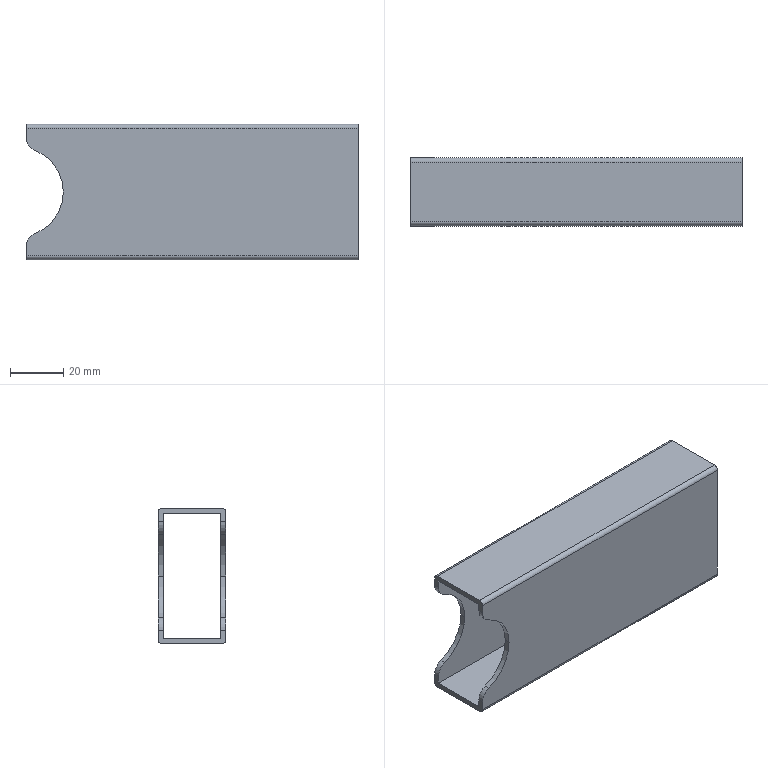Part | NX | features BREP 1 | 1 solid | 23 faces | box 124.206 x 25.4 x 50.8 mm | volume 33883 mm3 | cylinder 12 | plane 11 | commonest cylinder face diameters 3.175 x4 10.16 x4 33.528 x4
STEP:
#1=CARTESIAN_POINT('',(0.,12.7,-23.812));
#2=VERTEX_POINT('',#1);
#3=CARTESIAN_POINT('',(0.,12.7,-20.375));
#4=VERTEX_POINT('',#3);
#5=CARTESIAN_POINT('',(0.,12.7,-23.812));
#6=DIRECTION('',(0.,0.,1.));
#7=VECTOR('',#6,1000.);
#8=LINE('',#5,#7);
#9=EDGE_CURVE('',#2,#4,#8,.T.);
#10=ORIENTED_EDGE('',*,*,#9,.F.);
#11=CARTESIAN_POINT('',(0.,11.113,-25.4));
#12=VERTEX_POINT('',#11);
#13=CARTESIAN_POINT('',(0.,11.113,-23.812));
#14=DIRECTION('',(-1.,0.,0.));
#15=DIRECTION('',(0.,1.,0.));
#16=AXIS2_PLACEMENT_3D('',#13,#14,#15);
#17=CIRCLE('',#16,1.587);
#18=EDGE_CURVE('',#2,#12,#17,.T.);
#19=ORIENTED_EDGE('',*,*,#18,.T.);
#20=CARTESIAN_POINT('',(0.,-11.113,-25.4));
#21=VERTEX_POINT('',#20);
#22=CARTESIAN_POINT('',(0.,-11.113,-25.4));
#23=DIRECTION('',(0.,1.,0.));
#24=VECTOR('',#23,1000.);
#25=LINE('',#22,#24);
#26=EDGE_CURVE('',#21,#12,#25,.T.);
#27=ORIENTED_EDGE('',*,*,#26,.F.);
#28=CARTESIAN_POINT('',(0.,-12.7,-23.812));
#29=VERTEX_POINT('',#28);
#30=CARTESIAN_POINT('',(0.,-11.113,-23.812));
#31=DIRECTION('',(-1.,0.,0.));
#32=DIRECTION('',(0.,0.,-1.));
#33=AXIS2_PLACEMENT_3D('',#30,#31,#32);
#34=CIRCLE('',#33,1.587);
#35=EDGE_CURVE('',#21,#29,#34,.T.);
#36=ORIENTED_EDGE('',*,*,#35,.T.);
#37=CARTESIAN_POINT('',(0.,-12.7,-20.375));
#38=VERTEX_POINT('',#37);
#39=CARTESIAN_POINT('',(0.,-12.7,-20.375));
#40=DIRECTION('',(0.,0.,-1.));
#41=VECTOR('',#40,1000.);
#42=LINE('',#39,#41);
#43=EDGE_CURVE('',#38,#29,#42,.T.);
#44=ORIENTED_EDGE('',*,*,#43,.F.);
#45=CARTESIAN_POINT('',(0.,-10.719,-20.375));
#46=VERTEX_POINT('',#45);
#47=CARTESIAN_POINT('',(0.,-12.7,-20.375));
#48=DIRECTION('',(0.,1.,0.));
#49=VECTOR('',#48,1000.);
#50=LINE('',#47,#49);
#51=EDGE_CURVE('',#38,#46,#50,.T.);
#52=ORIENTED_EDGE('',*,*,#51,.T.);
#53=CARTESIAN_POINT('',(0.,-10.719,-23.419));
#54=VERTEX_POINT('',#53);
#55=CARTESIAN_POINT('',(0.,-10.719,-23.419));
#56=DIRECTION('',(0.,0.,1.));
#57=VECTOR('',#56,1000.);
#58=LINE('',#55,#57);
#59=EDGE_CURVE('',#54,#46,#58,.T.);
#60=ORIENTED_EDGE('',*,*,#59,.F.);
#61=CARTESIAN_POINT('',(0.,10.719,-23.419));
#62=VERTEX_POINT('',#61);
#63=CARTESIAN_POINT('',(0.,10.719,-23.419));
#64=DIRECTION('',(0.,-1.,0.));
#65=VECTOR('',#64,1000.);
#66=LINE('',#63,#65);
#67=EDGE_CURVE('',#62,#54,#66,.T.);
#68=ORIENTED_EDGE('',*,*,#67,.F.);
#69=CARTESIAN_POINT('',(0.,10.719,-20.375));
#70=VERTEX_POINT('',#69);
#71=CARTESIAN_POINT('',(0.,10.719,-20.375));
#72=DIRECTION('',(0.,0.,-1.));
#73=VECTOR('',#72,1000.);
#74=LINE('',#71,#73);
#75=EDGE_CURVE('',#70,#62,#74,.T.);
#76=ORIENTED_EDGE('',*,*,#75,.F.);
#77=CARTESIAN_POINT('',(0.,10.719,-20.375));
#78=DIRECTION('',(0.,1.,0.));
#79=VECTOR('',#78,1000.);
#80=LINE('',#77,#79);
#81=EDGE_CURVE('',#70,#4,#80,.T.);
#82=ORIENTED_EDGE('',*,*,#81,.T.);
#83=EDGE_LOOP('',(#10,#19,#27,#36,#44,#52,#60,#68,#76,#82));
#84=FACE_BOUND('',#83,.T.);
#85=CARTESIAN_POINT('',(0.,0.,0.));
#86=DIRECTION('',(1.,0.,0.));
#87=DIRECTION('',(0.,1.,0.));
#88=AXIS2_PLACEMENT_3D('',#85,#86,#87);
#89=PLANE('',#88);
#90=ADVANCED_FACE('',(#84),#89,.F.);
#91=CARTESIAN_POINT('',(0.,-12.7,23.812));
#92=VERTEX_POINT('',#91);
#93=CARTESIAN_POINT('',(0.,-12.7,20.375));
#94=VERTEX_POINT('',#93);
#95=CARTESIAN_POINT('',(0.,-12.7,23.812));
#96=DIRECTION('',(0.,0.,-1.));
#97=VECTOR('',#96,1000.);
#98=LINE('',#95,#97);
#99=EDGE_CURVE('',#92,#94,#98,.T.);
#100=ORIENTED_EDGE('',*,*,#99,.F.);
#101=CARTESIAN_POINT('',(0.,-11.113,25.4));
#102=VERTEX_POINT('',#101);
#103=CARTESIAN_POINT('',(0.,-11.113,23.812));
#104=DIRECTION('',(-1.,0.,0.));
#105=DIRECTION('',(0.,-1.,0.));
#106=AXIS2_PLACEMENT_3D('',#103,#104,#105);
#107=CIRCLE('',#106,1.587);
#108=EDGE_CURVE('',#92,#102,#107,.T.);
#109=ORIENTED_EDGE('',*,*,#108,.T.);
#110=CARTESIAN_POINT('',(0.,11.113,25.4));
#111=VERTEX_POINT('',#110);
#112=CARTESIAN_POINT('',(0.,11.113,25.4));
#113=DIRECTION('',(0.,-1.,0.));
#114=VECTOR('',#113,1000.);
#115=LINE('',#112,#114);
#116=EDGE_CURVE('',#111,#102,#115,.T.);
#117=ORIENTED_EDGE('',*,*,#116,.F.);
#118=CARTESIAN_POINT('',(0.,12.7,23.812));
#119=VERTEX_POINT('',#118);
#120=CARTESIAN_POINT('',(0.,11.113,23.812));
#121=DIRECTION('',(-1.,0.,0.));
#122=DIRECTION('',(0.,0.,1.));
#123=AXIS2_PLACEMENT_3D('',#120,#121,#122);
#124=CIRCLE('',#123,1.587);
#125=EDGE_CURVE('',#111,#119,#124,.T.);
#126=ORIENTED_EDGE('',*,*,#125,.T.);
#127=CARTESIAN_POINT('',(0.,12.7,20.375));
#128=VERTEX_POINT('',#127);
#129=CARTESIAN_POINT('',(0.,12.7,20.375));
#130=DIRECTION('',(0.,0.,1.));
#131=VECTOR('',#130,1000.);
#132=LINE('',#129,#131);
#133=EDGE_CURVE('',#128,#119,#132,.T.);
#134=ORIENTED_EDGE('',*,*,#133,.F.);
#135=CARTESIAN_POINT('',(0.,10.719,20.375));
#136=VERTEX_POINT('',#135);
#137=CARTESIAN_POINT('',(0.,12.7,20.375));
#138=DIRECTION('',(0.,-1.,0.));
#139=VECTOR('',#138,1000.);
#140=LINE('',#137,#139);
#141=EDGE_CURVE('',#128,#136,#140,.T.);
#142=ORIENTED_EDGE('',*,*,#141,.T.);
#143=CARTESIAN_POINT('',(0.,10.719,23.419));
#144=VERTEX_POINT('',#143);
#145=CARTESIAN_POINT('',(0.,10.719,23.419));
#146=DIRECTION('',(0.,0.,-1.));
#147=VECTOR('',#146,1000.);
#148=LINE('',#145,#147);
#149=EDGE_CURVE('',#144,#136,#148,.T.);
#150=ORIENTED_EDGE('',*,*,#149,.F.);
#151=CARTESIAN_POINT('',(0.,-10.719,23.419));
#152=VERTEX_POINT('',#151);
#153=CARTESIAN_POINT('',(0.,-10.719,23.419));
#154=DIRECTION('',(0.,1.,0.));
#155=VECTOR('',#154,1000.);
#156=LINE('',#153,#155);
#157=EDGE_CURVE('',#152,#144,#156,.T.);
#158=ORIENTED_EDGE('',*,*,#157,.F.);
#159=CARTESIAN_POINT('',(0.,-10.719,20.375));
#160=VERTEX_POINT('',#159);
#161=CARTESIAN_POINT('',(0.,-10.719,20.375));
#162=DIRECTION('',(0.,0.,1.));
#163=VECTOR('',#162,1000.);
#164=LINE('',#161,#163);
#165=EDGE_CURVE('',#160,#152,#164,.T.);
#166=ORIENTED_EDGE('',*,*,#165,.F.);
#167=CARTESIAN_POINT('',(0.,-10.719,20.375));
#168=DIRECTION('',(0.,-1.,0.));
#169=VECTOR('',#168,1000.);
#170=LINE('',#167,#169);
#171=EDGE_CURVE('',#160,#94,#170,.T.);
#172=ORIENTED_EDGE('',*,*,#171,.T.);
#173=EDGE_LOOP('',(#100,#109,#117,#126,#134,#142,#150,#158,#166,#172));
#174=FACE_BOUND('',#173,.T.);
#175=CARTESIAN_POINT('',(0.,0.,0.));
#176=DIRECTION('',(1.,0.,0.));
#177=DIRECTION('',(0.,1.,0.));
#178=AXIS2_PLACEMENT_3D('',#175,#176,#177);
#179=PLANE('',#178);
#180=ADVANCED_FACE('',(#174),#179,.F.);
#181=CARTESIAN_POINT('',(3.249,10.719,-15.637));
#182=VERTEX_POINT('',#181);
#183=CARTESIAN_POINT('',(5.08,10.719,-20.375));
#184=DIRECTION('',(0.,-1.,0.));
#185=DIRECTION('',(-0.3605,0.,0.9328));
#186=AXIS2_PLACEMENT_3D('',#183,#184,#185);
#187=CIRCLE('',#186,5.08);
#188=EDGE_CURVE('',#182,#70,#187,.T.);
#189=ORIENTED_EDGE('',*,*,#188,.F.);
#190=CARTESIAN_POINT('',(3.249,12.7,-15.637));
#191=VERTEX_POINT('',#190);
#192=CARTESIAN_POINT('',(3.249,10.719,-15.637));
#193=DIRECTION('',(0.,1.,0.));
#194=VECTOR('',#193,1000.);
#195=LINE('',#192,#194);
#196=EDGE_CURVE('',#182,#191,#195,.T.);
#197=ORIENTED_EDGE('',*,*,#196,.T.);
#198=CARTESIAN_POINT('',(5.08,12.7,-20.375));
#199=DIRECTION('',(0.,1.,0.));
#200=DIRECTION('',(-1.,0.,0.));
#201=AXIS2_PLACEMENT_3D('',#198,#199,#200);
#202=CIRCLE('',#201,5.08);
#203=EDGE_CURVE('',#4,#191,#202,.T.);
#204=ORIENTED_EDGE('',*,*,#203,.F.);
#205=ORIENTED_EDGE('',*,*,#81,.F.);
#206=EDGE_LOOP('',(#189,#197,#204,#205));
#207=FACE_BOUND('',#206,.T.);
#208=CARTESIAN_POINT('',(5.08,-12.883,-20.375));
#209=DIRECTION('',(0.,1.,0.));
#210=DIRECTION('',(-1.,0.,0.));
#211=AXIS2_PLACEMENT_3D('',#208,#209,#210);
#212=CYLINDRICAL_SURFACE('',#211,5.08);
#213=ADVANCED_FACE('',(#207),#212,.T.);
#214=CARTESIAN_POINT('',(3.249,12.7,15.637));
#215=VERTEX_POINT('',#214);
#216=CARTESIAN_POINT('',(13.97,12.7,0.));
#217=VERTEX_POINT('',#216);
#218=CARTESIAN_POINT('',(-2.794,12.7,0.));
#219=DIRECTION('',(0.,1.,0.));
#220=DIRECTION('',(0.3605,0.,0.9328));
#221=AXIS2_PLACEMENT_3D('',#218,#219,#220);
#222=CIRCLE('',#221,16.764);
#223=EDGE_CURVE('',#215,#217,#222,.T.);
#224=ORIENTED_EDGE('',*,*,#223,.F.);
#225=CARTESIAN_POINT('',(5.08,12.7,20.375));
#226=DIRECTION('',(0.,1.,0.));
#227=DIRECTION('',(-0.3605,0.,-0.9328));
#228=AXIS2_PLACEMENT_3D('',#225,#226,#227);
#229=CIRCLE('',#228,5.08);
#230=EDGE_CURVE('',#215,#128,#229,.T.);
#231=ORIENTED_EDGE('',*,*,#230,.T.);
#232=ORIENTED_EDGE('',*,*,#133,.T.);
#233=CARTESIAN_POINT('',(124.206,12.7,23.812));
#234=VERTEX_POINT('',#233);
#235=CARTESIAN_POINT('',(124.206,12.7,23.812));
#236=DIRECTION('',(-1.,0.,0.));
#237=VECTOR('',#236,1000.);
#238=LINE('',#235,#237);
#239=EDGE_CURVE('',#234,#119,#238,.T.);
#240=ORIENTED_EDGE('',*,*,#239,.F.);
#241=CARTESIAN_POINT('',(124.206,12.7,-23.812));
#242=VERTEX_POINT('',#241);
#243=CARTESIAN_POINT('',(124.206,12.7,-23.812));
#244=DIRECTION('',(0.,0.,1.));
#245=VECTOR('',#244,1000.);
#246=LINE('',#243,#245);
#247=EDGE_CURVE('',#242,#234,#246,.T.);
#248=ORIENTED_EDGE('',*,*,#247,.F.);
#249=CARTESIAN_POINT('',(124.206,12.7,-23.812));
#250=DIRECTION('',(-1.,0.,0.));
#251=VECTOR('',#250,1000.);
#252=LINE('',#249,#251);
#253=EDGE_CURVE('',#242,#2,#252,.T.);
#254=ORIENTED_EDGE('',*,*,#253,.T.);
#255=ORIENTED_EDGE('',*,*,#9,.T.);
#256=ORIENTED_EDGE('',*,*,#203,.T.);
#257=CARTESIAN_POINT('',(-2.794,12.7,0.));
#258=DIRECTION('',(0.,1.,0.));
#259=DIRECTION('',(0.3605,0.,0.9328));
#260=AXIS2_PLACEMENT_3D('',#257,#258,#259);
#261=CIRCLE('',#260,16.764);
#262=EDGE_CURVE('',#217,#191,#261,.T.);
#263=ORIENTED_EDGE('',*,*,#262,.F.);
#264=EDGE_LOOP('',(#224,#231,#232,#240,#248,#254,#255,#256,#263));
#265=FACE_BOUND('',#264,.T.);
#266=CARTESIAN_POINT('',(0.,12.7,-25.4));
#267=DIRECTION('',(0.,1.,0.));
#268=DIRECTION('',(1.,0.,0.));
#269=AXIS2_PLACEMENT_3D('',#266,#267,#268);
#270=PLANE('',#269);
#271=ADVANCED_FACE('',(#265),#270,.T.);
#272=CARTESIAN_POINT('',(124.206,11.113,-25.4));
#273=VERTEX_POINT('',#272);
#274=CARTESIAN_POINT('',(124.206,11.113,-23.812));
#275=DIRECTION('',(1.,0.,0.));
#276=DIRECTION('',(0.,0.,-1.));
#277=AXIS2_PLACEMENT_3D('',#274,#275,#276);
#278=CIRCLE('',#277,1.587);
#279=EDGE_CURVE('',#273,#242,#278,.T.);
#280=ORIENTED_EDGE('',*,*,#279,.F.);
#281=CARTESIAN_POINT('',(124.206,11.113,-25.4));
#282=DIRECTION('',(-1.,0.,0.));
#283=VECTOR('',#282,1000.);
#284=LINE('',#281,#283);
#285=EDGE_CURVE('',#273,#12,#284,.T.);
#286=ORIENTED_EDGE('',*,*,#285,.T.);
#287=ORIENTED_EDGE('',*,*,#18,.F.);
#288=ORIENTED_EDGE('',*,*,#253,.F.);
#289=EDGE_LOOP('',(#280,#286,#287,#288));
#290=FACE_BOUND('',#289,.T.);
#291=CARTESIAN_POINT('',(124.42,11.113,-23.812));
#292=DIRECTION('',(-1.,0.,0.));
#293=DIRECTION('',(0.,1.,0.));
#294=AXIS2_PLACEMENT_3D('',#291,#292,#293);
#295=CYLINDRICAL_SURFACE('',#294,1.587);
#296=ADVANCED_FACE('',(#290),#295,.T.);
#297=CARTESIAN_POINT('',(124.206,-11.113,-25.4));
#298=VERTEX_POINT('',#297);
#299=CARTESIAN_POINT('',(124.206,-11.113,-25.4));
#300=DIRECTION('',(0.,1.,0.));
#301=VECTOR('',#300,1000.);
#302=LINE('',#299,#301);
#303=EDGE_CURVE('',#298,#273,#302,.T.);
#304=ORIENTED_EDGE('',*,*,#303,.F.);
#305=CARTESIAN_POINT('',(124.206,-11.113,-25.4));
#306=DIRECTION('',(-1.,0.,0.));
#307=VECTOR('',#306,1000.);
#308=LINE('',#305,#307);
#309=EDGE_CURVE('',#298,#21,#308,.T.);
#310=ORIENTED_EDGE('',*,*,#309,.T.);
#311=ORIENTED_EDGE('',*,*,#26,.T.);
#312=ORIENTED_EDGE('',*,*,#285,.F.);
#313=EDGE_LOOP('',(#304,#310,#311,#312));
#314=FACE_BOUND('',#313,.T.);
#315=CARTESIAN_POINT('',(0.,-12.7,-25.4));
#316=DIRECTION('',(0.,0.,-1.));
#317=DIRECTION('',(0.,-1.,0.));
#318=AXIS2_PLACEMENT_3D('',#315,#316,#317);
#319=PLANE('',#318);
#320=ADVANCED_FACE('',(#314),#319,.T.);
#321=CARTESIAN_POINT('',(124.206,-12.7,-23.812));
#322=VERTEX_POINT('',#321);
#323=CARTESIAN_POINT('',(124.206,-11.113,-23.812));
#324=DIRECTION('',(1.,0.,0.));
#325=DIRECTION('',(0.,-1.,0.));
#326=AXIS2_PLACEMENT_3D('',#323,#324,#325);
#327=CIRCLE('',#326,1.587);
#328=EDGE_CURVE('',#322,#298,#327,.T.);
#329=ORIENTED_EDGE('',*,*,#328,.F.);
#330=CARTESIAN_POINT('',(124.206,-12.7,-23.812));
#331=DIRECTION('',(-1.,0.,0.));
#332=VECTOR('',#331,1000.);
#333=LINE('',#330,#332);
#334=EDGE_CURVE('',#322,#29,#333,.T.);
#335=ORIENTED_EDGE('',*,*,#334,.T.);
#336=ORIENTED_EDGE('',*,*,#35,.F.);
#337=ORIENTED_EDGE('',*,*,#309,.F.);
#338=EDGE_LOOP('',(#329,#335,#336,#337));
#339=FACE_BOUND('',#338,.T.);
#340=CARTESIAN_POINT('',(124.42,-11.113,-23.812));
#341=DIRECTION('',(-1.,0.,0.));
#342=DIRECTION('',(0.,0.,-1.));
#343=AXIS2_PLACEMENT_3D('',#340,#341,#342);
#344=CYLINDRICAL_SURFACE('',#343,1.587);
#345=ADVANCED_FACE('',(#339),#344,.T.);
#346=ORIENTED_EDGE('',*,*,#43,.T.);
#347=ORIENTED_EDGE('',*,*,#334,.F.);
#348=CARTESIAN_POINT('',(124.206,-12.7,23.812));
#349=VERTEX_POINT('',#348);
#350=CARTESIAN_POINT('',(124.206,-12.7,23.812));
#351=DIRECTION('',(0.,0.,-1.));
#352=VECTOR('',#351,1000.);
#353=LINE('',#350,#352);
#354=EDGE_CURVE('',#349,#322,#353,.T.);
#355=ORIENTED_EDGE('',*,*,#354,.F.);
#356=CARTESIAN_POINT('',(124.206,-12.7,23.812));
#357=DIRECTION('',(-1.,0.,0.));
#358=VECTOR('',#357,1000.);
#359=LINE('',#356,#358);
#360=EDGE_CURVE('',#349,#92,#359,.T.);
#361=ORIENTED_EDGE('',*,*,#360,.T.);
#362=ORIENTED_EDGE('',*,*,#99,.T.);
#363=CARTESIAN_POINT('',(3.249,-12.7,15.637));
#364=VERTEX_POINT('',#363);
#365=CARTESIAN_POINT('',(5.08,-12.7,20.375));
#366=DIRECTION('',(0.,-1.,0.));
#367=DIRECTION('',(-1.,0.,0.));
#368=AXIS2_PLACEMENT_3D('',#365,#366,#367);
#369=CIRCLE('',#368,5.08);
#370=EDGE_CURVE('',#94,#364,#369,.T.);
#371=ORIENTED_EDGE('',*,*,#370,.T.);
#372=CARTESIAN_POINT('',(13.97,-12.7,0.));
#373=VERTEX_POINT('',#372);
#374=CARTESIAN_POINT('',(-2.794,-12.7,0.));
#375=DIRECTION('',(0.,1.,0.));
#376=DIRECTION('',(0.3605,0.,0.9328));
#377=AXIS2_PLACEMENT_3D('',#374,#375,#376);
#378=CIRCLE('',#377,16.764);
#379=EDGE_CURVE('',#364,#373,#378,.T.);
#380=ORIENTED_EDGE('',*,*,#379,.T.);
#381=CARTESIAN_POINT('',(3.249,-12.7,-15.637));
#382=VERTEX_POINT('',#381);
#383=CARTESIAN_POINT('',(-2.794,-12.7,0.));
#384=DIRECTION('',(0.,1.,0.));
#385=DIRECTION('',(0.3605,0.,0.9328));
#386=AXIS2_PLACEMENT_3D('',#383,#384,#385);
#387=CIRCLE('',#386,16.764);
#388=EDGE_CURVE('',#373,#382,#387,.T.);
#389=ORIENTED_EDGE('',*,*,#388,.T.);
#390=CARTESIAN_POINT('',(5.08,-12.7,-20.375));
#391=DIRECTION('',(0.,-1.,0.));
#392=DIRECTION('',(-0.3605,0.,0.9328));
#393=AXIS2_PLACEMENT_3D('',#390,#391,#392);
#394=CIRCLE('',#393,5.08);
#395=EDGE_CURVE('',#382,#38,#394,.T.);
#396=ORIENTED_EDGE('',*,*,#395,.T.);
#397=EDGE_LOOP('',(#346,#347,#355,#361,#362,#371,#380,#389,#396));
#398=FACE_BOUND('',#397,.T.);
#399=CARTESIAN_POINT('',(0.,-12.7,25.4));
#400=DIRECTION('',(0.,-1.,0.));
#401=DIRECTION('',(0.,0.,-1.));
#402=AXIS2_PLACEMENT_3D('',#399,#400,#401);
#403=PLANE('',#402);
#404=ADVANCED_FACE('',(#398),#403,.T.);
#405=ORIENTED_EDGE('',*,*,#395,.F.);
#406=CARTESIAN_POINT('',(3.249,-10.719,-15.637));
#407=VERTEX_POINT('',#406);
#408=CARTESIAN_POINT('',(3.249,-12.7,-15.637));
#409=DIRECTION('',(0.,1.,0.));
#410=VECTOR('',#409,1000.);
#411=LINE('',#408,#410);
#412=EDGE_CURVE('',#382,#407,#411,.T.);
#413=ORIENTED_EDGE('',*,*,#412,.T.);
#414=CARTESIAN_POINT('',(5.08,-10.719,-20.375));
#415=DIRECTION('',(0.,1.,0.));
#416=DIRECTION('',(-1.,0.,0.));
#417=AXIS2_PLACEMENT_3D('',#414,#415,#416);
#418=CIRCLE('',#417,5.08);
#419=EDGE_CURVE('',#46,#407,#418,.T.);
#420=ORIENTED_EDGE('',*,*,#419,.F.);
#421=ORIENTED_EDGE('',*,*,#51,.F.);
#422=EDGE_LOOP('',(#405,#413,#420,#421));
#423=FACE_BOUND('',#422,.T.);
#424=CARTESIAN_POINT('',(5.08,-12.883,-20.375));
#425=DIRECTION('',(0.,1.,0.));
#426=DIRECTION('',(-1.,0.,0.));
#427=AXIS2_PLACEMENT_3D('',#424,#425,#426);
#428=CYLINDRICAL_SURFACE('',#427,5.08);
#429=ADVANCED_FACE('',(#423),#428,.T.);
#430=CARTESIAN_POINT('',(3.249,-10.719,15.637));
#431=VERTEX_POINT('',#430);
#432=CARTESIAN_POINT('',(13.97,-10.719,0.));
#433=VERTEX_POINT('',#432);
#434=CARTESIAN_POINT('',(-2.794,-10.719,0.));
#435=DIRECTION('',(0.,1.,0.));
#436=DIRECTION('',(0.3605,0.,0.9328));
#437=AXIS2_PLACEMENT_3D('',#434,#435,#436);
#438=CIRCLE('',#437,16.764);
#439=EDGE_CURVE('',#431,#433,#438,.T.);
#440=ORIENTED_EDGE('',*,*,#439,.F.);
#441=CARTESIAN_POINT('',(5.08,-10.719,20.375));
#442=DIRECTION('',(0.,1.,0.));
#443=DIRECTION('',(-0.3605,0.,-0.9328));
#444=AXIS2_PLACEMENT_3D('',#441,#442,#443);
#445=CIRCLE('',#444,5.08);
#446=EDGE_CURVE('',#431,#160,#445,.T.);
#447=ORIENTED_EDGE('',*,*,#446,.T.);
#448=ORIENTED_EDGE('',*,*,#165,.T.);
#449=CARTESIAN_POINT('',(124.206,-10.719,23.419));
#450=VERTEX_POINT('',#449);
#451=CARTESIAN_POINT('',(0.,-10.719,23.419));
#452=DIRECTION('',(1.,0.,0.));
#453=VECTOR('',#452,1000.);
#454=LINE('',#451,#453);
#455=EDGE_CURVE('',#152,#450,#454,.T.);
#456=ORIENTED_EDGE('',*,*,#455,.T.);
#457=CARTESIAN_POINT('',(124.206,-10.719,-23.419));
#458=VERTEX_POINT('',#457);
#459=CARTESIAN_POINT('',(124.206,-10.719,-23.419));
#460=DIRECTION('',(0.,0.,1.));
#461=VECTOR('',#460,1000.);
#462=LINE('',#459,#461);
#463=EDGE_CURVE('',#458,#450,#462,.T.);
#464=ORIENTED_EDGE('',*,*,#463,.F.);
#465=CARTESIAN_POINT('',(0.,-10.719,-23.419));
#466=DIRECTION('',(1.,0.,0.));
#467=VECTOR('',#466,1000.);
#468=LINE('',#465,#467);
#469=EDGE_CURVE('',#54,#458,#468,.T.);
#470=ORIENTED_EDGE('',*,*,#469,.F.);
#471=ORIENTED_EDGE('',*,*,#59,.T.);
#472=ORIENTED_EDGE('',*,*,#419,.T.);
#473=CARTESIAN_POINT('',(-2.794,-10.719,0.));
#474=DIRECTION('',(0.,1.,0.));
#475=DIRECTION('',(0.3605,0.,0.9328));
#476=AXIS2_PLACEMENT_3D('',#473,#474,#475);
#477=CIRCLE('',#476,16.764);
#478=EDGE_CURVE('',#433,#407,#477,.T.);
#479=ORIENTED_EDGE('',*,*,#478,.F.);
#480=EDGE_LOOP('',(#440,#447,#448,#456,#464,#470,#471,#472,#479));
#481=FACE_BOUND('',#480,.T.);
#482=CARTESIAN_POINT('',(0.,-10.719,-23.419));
#483=DIRECTION('',(0.,1.,0.));
#484=DIRECTION('',(1.,0.,0.));
#485=AXIS2_PLACEMENT_3D('',#482,#483,#484);
#486=PLANE('',#485);
#487=ADVANCED_FACE('',(#481),#486,.T.);
#488=ORIENTED_EDGE('',*,*,#469,.T.);
#489=CARTESIAN_POINT('',(124.206,10.719,-23.419));
#490=VERTEX_POINT('',#489);
#491=CARTESIAN_POINT('',(124.206,10.719,-23.419));
#492=DIRECTION('',(0.,-1.,0.));
#493=VECTOR('',#492,1000.);
#494=LINE('',#491,#493);
#495=EDGE_CURVE('',#490,#458,#494,.T.);
#496=ORIENTED_EDGE('',*,*,#495,.F.);
#497=CARTESIAN_POINT('',(0.,10.719,-23.419));
#498=DIRECTION('',(1.,0.,0.));
#499=VECTOR('',#498,1000.);
#500=LINE('',#497,#499);
#501=EDGE_CURVE('',#62,#490,#500,.T.);
#502=ORIENTED_EDGE('',*,*,#501,.F.);
#503=ORIENTED_EDGE('',*,*,#67,.T.);
#504=EDGE_LOOP('',(#488,#496,#502,#503));
#505=FACE_BOUND('',#504,.T.);
#506=CARTESIAN_POINT('',(0.,10.719,-23.419));
#507=DIRECTION('',(0.,0.,1.));
#508=DIRECTION('',(1.,0.,0.));
#509=AXIS2_PLACEMENT_3D('',#506,#507,#508);
#510=PLANE('',#509);
#511=ADVANCED_FACE('',(#505),#510,.T.);
#512=ORIENTED_EDGE('',*,*,#75,.T.);
#513=ORIENTED_EDGE('',*,*,#501,.T.);
#514=CARTESIAN_POINT('',(124.206,10.719,23.419));
#515=VERTEX_POINT('',#514);
#516=CARTESIAN_POINT('',(124.206,10.719,23.419));
#517=DIRECTION('',(0.,0.,-1.));
#518=VECTOR('',#517,1000.);
#519=LINE('',#516,#518);
#520=EDGE_CURVE('',#515,#490,#519,.T.);
#521=ORIENTED_EDGE('',*,*,#520,.F.);
#522=CARTESIAN_POINT('',(0.,10.719,23.419));
#523=DIRECTION('',(1.,0.,0.));
#524=VECTOR('',#523,1000.);
#525=LINE('',#522,#524);
#526=EDGE_CURVE('',#144,#515,#525,.T.);
#527=ORIENTED_EDGE('',*,*,#526,.F.);
#528=ORIENTED_EDGE('',*,*,#149,.T.);
#529=CARTESIAN_POINT('',(3.249,10.719,15.637));
#530=VERTEX_POINT('',#529);
#531=CARTESIAN_POINT('',(5.08,10.719,20.375));
#532=DIRECTION('',(0.,-1.,0.));
#533=DIRECTION('',(-1.,0.,0.));
#534=AXIS2_PLACEMENT_3D('',#531,#532,#533);
#535=CIRCLE('',#534,5.08);
#536=EDGE_CURVE('',#136,#530,#535,.T.);
#537=ORIENTED_EDGE('',*,*,#536,.T.);
#538=CARTESIAN_POINT('',(13.97,10.719,0.));
#539=VERTEX_POINT('',#538);
#540=CARTESIAN_POINT('',(-2.794,10.719,0.));
#541=DIRECTION('',(0.,1.,0.));
#542=DIRECTION('',(0.3605,0.,0.9328));
#543=AXIS2_PLACEMENT_3D('',#540,#541,#542);
#544=CIRCLE('',#543,16.764);
#545=EDGE_CURVE('',#530,#539,#544,.T.);
#546=ORIENTED_EDGE('',*,*,#545,.T.);
#547=CARTESIAN_POINT('',(-2.794,10.719,0.));
#548=DIRECTION('',(0.,1.,0.));
#549=DIRECTION('',(0.3605,0.,0.9328));
#550=AXIS2_PLACEMENT_3D('',#547,#548,#549);
#551=CIRCLE('',#550,16.764);
#552=EDGE_CURVE('',#539,#182,#551,.T.);
#553=ORIENTED_EDGE('',*,*,#552,.T.);
#554=ORIENTED_EDGE('',*,*,#188,.T.);
#555=EDGE_LOOP('',(#512,#513,#521,#527,#528,#537,#546,#553,#554));
#556=FACE_BOUND('',#555,.T.);
#557=CARTESIAN_POINT('',(0.,10.719,23.419));
#558=DIRECTION('',(0.,-1.,0.));
#559=DIRECTION('',(0.,0.,-1.));
#560=AXIS2_PLACEMENT_3D('',#557,#558,#559);
#561=PLANE('',#560);
#562=ADVANCED_FACE('',(#556),#561,.T.);
#563=CARTESIAN_POINT('',(13.97,15.24,0.));
#564=DIRECTION('',(0.,1.,0.));
#565=VECTOR('',#564,1000.);
#566=LINE('',#563,#565);
#567=EDGE_CURVE('',#539,#217,#566,.T.);
#568=ORIENTED_EDGE('',*,*,#567,.F.);
#569=ORIENTED_EDGE('',*,*,#545,.F.);
#570=CARTESIAN_POINT('',(3.249,12.7,15.637));
#571=DIRECTION('',(0.,-1.,0.));
#572=VECTOR('',#571,1000.);
#573=LINE('',#570,#572);
#574=EDGE_CURVE('',#215,#530,#573,.T.);
#575=ORIENTED_EDGE('',*,*,#574,.F.);
#576=ORIENTED_EDGE('',*,*,#223,.T.);
#577=EDGE_LOOP('',(#568,#569,#575,#576));
#578=FACE_BOUND('',#577,.T.);
#579=CARTESIAN_POINT('',(-2.794,15.24,0.));
#580=DIRECTION('',(0.,1.,0.));
#581=DIRECTION('',(1.,0.,0.));
#582=AXIS2_PLACEMENT_3D('',#579,#580,#581);
#583=CYLINDRICAL_SURFACE('',#582,16.764);
#584=ADVANCED_FACE('',(#578),#583,.F.);
#585=CARTESIAN_POINT('',(13.97,15.24,0.));
#586=DIRECTION('',(0.,1.,0.));
#587=VECTOR('',#586,1000.);
#588=LINE('',#585,#587);
#589=EDGE_CURVE('',#373,#433,#588,.T.);
#590=ORIENTED_EDGE('',*,*,#589,.F.);
#591=ORIENTED_EDGE('',*,*,#379,.F.);
#592=CARTESIAN_POINT('',(3.249,-10.719,15.637));
#593=DIRECTION('',(0.,-1.,0.));
#594=VECTOR('',#593,1000.);
#595=LINE('',#592,#594);
#596=EDGE_CURVE('',#431,#364,#595,.T.);
#597=ORIENTED_EDGE('',*,*,#596,.F.);
#598=ORIENTED_EDGE('',*,*,#439,.T.);
#599=EDGE_LOOP('',(#590,#591,#597,#598));
#600=FACE_BOUND('',#599,.T.);
#601=CARTESIAN_POINT('',(-2.794,15.24,0.));
#602=DIRECTION('',(0.,1.,0.));
#603=DIRECTION('',(1.,0.,0.));
#604=AXIS2_PLACEMENT_3D('',#601,#602,#603);
#605=CYLINDRICAL_SURFACE('',#604,16.764);
#606=ADVANCED_FACE('',(#600),#605,.F.);
#607=ORIENTED_EDGE('',*,*,#230,.F.);
#608=ORIENTED_EDGE('',*,*,#574,.T.);
#609=ORIENTED_EDGE('',*,*,#536,.F.);
#610=ORIENTED_EDGE('',*,*,#141,.F.);
#611=EDGE_LOOP('',(#607,#608,#609,#610));
#612=FACE_BOUND('',#611,.T.);
#613=CARTESIAN_POINT('',(5.08,12.92,20.375));
#614=DIRECTION('',(0.,-1.,0.));
#615=DIRECTION('',(-1.,0.,0.));
#616=AXIS2_PLACEMENT_3D('',#613,#614,#615);
#617=CYLINDRICAL_SURFACE('',#616,5.08);
#618=ADVANCED_FACE('',(#612),#617,.T.);
#619=ORIENTED_EDGE('',*,*,#446,.F.);
#620=ORIENTED_EDGE('',*,*,#596,.T.);
#621=ORIENTED_EDGE('',*,*,#370,.F.);
#622=ORIENTED_EDGE('',*,*,#171,.F.);
#623=EDGE_LOOP('',(#619,#620,#621,#622));
#624=FACE_BOUND('',#623,.T.);
#625=CARTESIAN_POINT('',(5.08,12.92,20.375));
#626=DIRECTION('',(0.,-1.,0.));
#627=DIRECTION('',(-1.,0.,0.));
#628=AXIS2_PLACEMENT_3D('',#625,#626,#627);
#629=CYLINDRICAL_SURFACE('',#628,5.08);
#630=ADVANCED_FACE('',(#624),#629,.T.);
#631=ORIENTED_EDGE('',*,*,#526,.T.);
#632=CARTESIAN_POINT('',(124.206,-10.719,23.419));
#633=DIRECTION('',(0.,1.,0.));
#634=VECTOR('',#633,1000.);
#635=LINE('',#632,#634);
#636=EDGE_CURVE('',#450,#515,#635,.T.);
#637=ORIENTED_EDGE('',*,*,#636,.F.);
#638=ORIENTED_EDGE('',*,*,#455,.F.);
#639=ORIENTED_EDGE('',*,*,#157,.T.);
#640=EDGE_LOOP('',(#631,#637,#638,#639));
#641=FACE_BOUND('',#640,.T.);
#642=CARTESIAN_POINT('',(0.,-10.719,23.419));
#643=DIRECTION('',(0.,0.,-1.));
#644=DIRECTION('',(0.,-1.,0.));
#645=AXIS2_PLACEMENT_3D('',#642,#643,#644);
#646=PLANE('',#645);
#647=ADVANCED_FACE('',(#641),#646,.T.);
#648=CARTESIAN_POINT('',(124.206,11.113,25.4));
#649=VERTEX_POINT('',#648);
#650=CARTESIAN_POINT('',(124.206,-11.113,25.4));
#651=VERTEX_POINT('',#650);
#652=CARTESIAN_POINT('',(124.206,11.113,25.4));
#653=DIRECTION('',(0.,-1.,0.));
#654=VECTOR('',#653,1000.);
#655=LINE('',#652,#654);
#656=EDGE_CURVE('',#649,#651,#655,.T.);
#657=ORIENTED_EDGE('',*,*,#656,.T.);
#658=CARTESIAN_POINT('',(124.206,-11.113,23.812));
#659=DIRECTION('',(1.,0.,0.));
#660=DIRECTION('',(0.,0.,1.));
#661=AXIS2_PLACEMENT_3D('',#658,#659,#660);
#662=CIRCLE('',#661,1.587);
#663=EDGE_CURVE('',#651,#349,#662,.T.);
#664=ORIENTED_EDGE('',*,*,#663,.T.);
#665=ORIENTED_EDGE('',*,*,#354,.T.);
#666=ORIENTED_EDGE('',*,*,#328,.T.);
#667=ORIENTED_EDGE('',*,*,#303,.T.);
#668=ORIENTED_EDGE('',*,*,#279,.T.);
#669=ORIENTED_EDGE('',*,*,#247,.T.);
#670=CARTESIAN_POINT('',(124.206,11.113,23.812));
#671=DIRECTION('',(1.,0.,0.));
#672=DIRECTION('',(0.,1.,0.));
#673=AXIS2_PLACEMENT_3D('',#670,#671,#672);
#674=CIRCLE('',#673,1.587);
#675=EDGE_CURVE('',#234,#649,#674,.T.);
#676=ORIENTED_EDGE('',*,*,#675,.T.);
#677=EDGE_LOOP('',(#657,#664,#665,#666,#667,#668,#669,#676));
#678=FACE_BOUND('',#677,.T.);
#679=ORIENTED_EDGE('',*,*,#463,.T.);
#680=ORIENTED_EDGE('',*,*,#636,.T.);
#681=ORIENTED_EDGE('',*,*,#520,.T.);
#682=ORIENTED_EDGE('',*,*,#495,.T.);
#683=EDGE_LOOP('',(#679,#680,#681,#682));
#684=FACE_BOUND('',#683,.T.);
#685=CARTESIAN_POINT('',(124.206,0.,0.));
#686=DIRECTION('',(1.,0.,0.));
#687=DIRECTION('',(0.,1.,0.));
#688=AXIS2_PLACEMENT_3D('',#685,#686,#687);
#689=PLANE('',#688);
#690=ADVANCED_FACE('',(#678,#684),#689,.T.);
#691=ORIENTED_EDGE('',*,*,#675,.F.);
#692=ORIENTED_EDGE('',*,*,#239,.T.);
#693=ORIENTED_EDGE('',*,*,#125,.F.);
#694=CARTESIAN_POINT('',(124.206,11.113,25.4));
#695=DIRECTION('',(-1.,0.,0.));
#696=VECTOR('',#695,1000.);
#697=LINE('',#694,#696);
#698=EDGE_CURVE('',#649,#111,#697,.T.);
#699=ORIENTED_EDGE('',*,*,#698,.F.);
#700=EDGE_LOOP('',(#691,#692,#693,#699));
#701=FACE_BOUND('',#700,.T.);
#702=CARTESIAN_POINT('',(124.42,11.113,23.812));
#703=DIRECTION('',(-1.,0.,0.));
#704=DIRECTION('',(0.,0.,1.));
#705=AXIS2_PLACEMENT_3D('',#702,#703,#704);
#706=CYLINDRICAL_SURFACE('',#705,1.587);
#707=ADVANCED_FACE('',(#701),#706,.T.);
#708=ORIENTED_EDGE('',*,*,#116,.T.);
#709=CARTESIAN_POINT('',(124.206,-11.113,25.4));
#710=DIRECTION('',(-1.,0.,0.));
#711=VECTOR('',#710,1000.);
#712=LINE('',#709,#711);
#713=EDGE_CURVE('',#651,#102,#712,.T.);
#714=ORIENTED_EDGE('',*,*,#713,.F.);
#715=ORIENTED_EDGE('',*,*,#656,.F.);
#716=ORIENTED_EDGE('',*,*,#698,.T.);
#717=EDGE_LOOP('',(#708,#714,#715,#716));
#718=FACE_BOUND('',#717,.T.);
#719=CARTESIAN_POINT('',(0.,12.7,25.4));
#720=DIRECTION('',(0.,0.,1.));
#721=DIRECTION('',(1.,0.,0.));
#722=AXIS2_PLACEMENT_3D('',#719,#720,#721);
#723=PLANE('',#722);
#724=ADVANCED_FACE('',(#718),#723,.T.);
#725=ORIENTED_EDGE('',*,*,#663,.F.);
#726=ORIENTED_EDGE('',*,*,#713,.T.);
#727=ORIENTED_EDGE('',*,*,#108,.F.);
#728=ORIENTED_EDGE('',*,*,#360,.F.);
#729=EDGE_LOOP('',(#725,#726,#727,#728));
#730=FACE_BOUND('',#729,.T.);
#731=CARTESIAN_POINT('',(124.42,-11.113,23.812));
#732=DIRECTION('',(-1.,0.,0.));
#733=DIRECTION('',(0.,-1.,0.));
#734=AXIS2_PLACEMENT_3D('',#731,#732,#733);
#735=CYLINDRICAL_SURFACE('',#734,1.587);
#736=ADVANCED_FACE('',(#730),#735,.T.);
#737=ORIENTED_EDGE('',*,*,#388,.F.);
#738=ORIENTED_EDGE('',*,*,#589,.T.);
#739=ORIENTED_EDGE('',*,*,#478,.T.);
#740=ORIENTED_EDGE('',*,*,#412,.F.);
#741=EDGE_LOOP('',(#737,#738,#739,#740));
#742=FACE_BOUND('',#741,.T.);
#743=CARTESIAN_POINT('',(-2.794,15.24,0.));
#744=DIRECTION('',(0.,1.,0.));
#745=DIRECTION('',(1.,0.,0.));
#746=AXIS2_PLACEMENT_3D('',#743,#744,#745);
#747=CYLINDRICAL_SURFACE('',#746,16.764);
#748=ADVANCED_FACE('',(#742),#747,.F.);
#749=ORIENTED_EDGE('',*,*,#552,.F.);
#750=ORIENTED_EDGE('',*,*,#567,.T.);
#751=ORIENTED_EDGE('',*,*,#262,.T.);
#752=ORIENTED_EDGE('',*,*,#196,.F.);
#753=EDGE_LOOP('',(#749,#750,#751,#752));
#754=FACE_BOUND('',#753,.T.);
#755=CARTESIAN_POINT('',(-2.794,15.24,0.));
#756=DIRECTION('',(0.,1.,0.));
#757=DIRECTION('',(1.,0.,0.));
#758=AXIS2_PLACEMENT_3D('',#755,#756,#757);
#759=CYLINDRICAL_SURFACE('',#758,16.764);
#760=ADVANCED_FACE('',(#754),#759,.F.);
#761=CLOSED_SHELL('',(#90,#180,#213,#271,#296,#320,#345,#404,#429,#487,#511,#562,#584,#606,#618,#630,#647,#690,#707,#724,#736,#748,#760));
#762=MANIFOLD_SOLID_BREP('',#761);
#763=(LENGTH_UNIT()NAMED_UNIT(*)SI_UNIT(.MILLI.,.METRE.));
#764=UNCERTAINTY_MEASURE_WITH_UNIT(LENGTH_MEASURE(0.00001),#763,'','');
#765=(NAMED_UNIT(*)PLANE_ANGLE_UNIT()SI_UNIT($,.RADIAN.));
#766=(NAMED_UNIT(*)SI_UNIT($,.STERADIAN.)SOLID_ANGLE_UNIT());
#767=(GEOMETRIC_REPRESENTATION_CONTEXT(3)GLOBAL_UNCERTAINTY_ASSIGNED_CONTEXT((#764))GLOBAL_UNIT_ASSIGNED_CONTEXT((#763,#765,#766))REPRESENTATION_CONTEXT('',''));
#768=ADVANCED_BREP_SHAPE_REPRESENTATION('',(#762),#767);